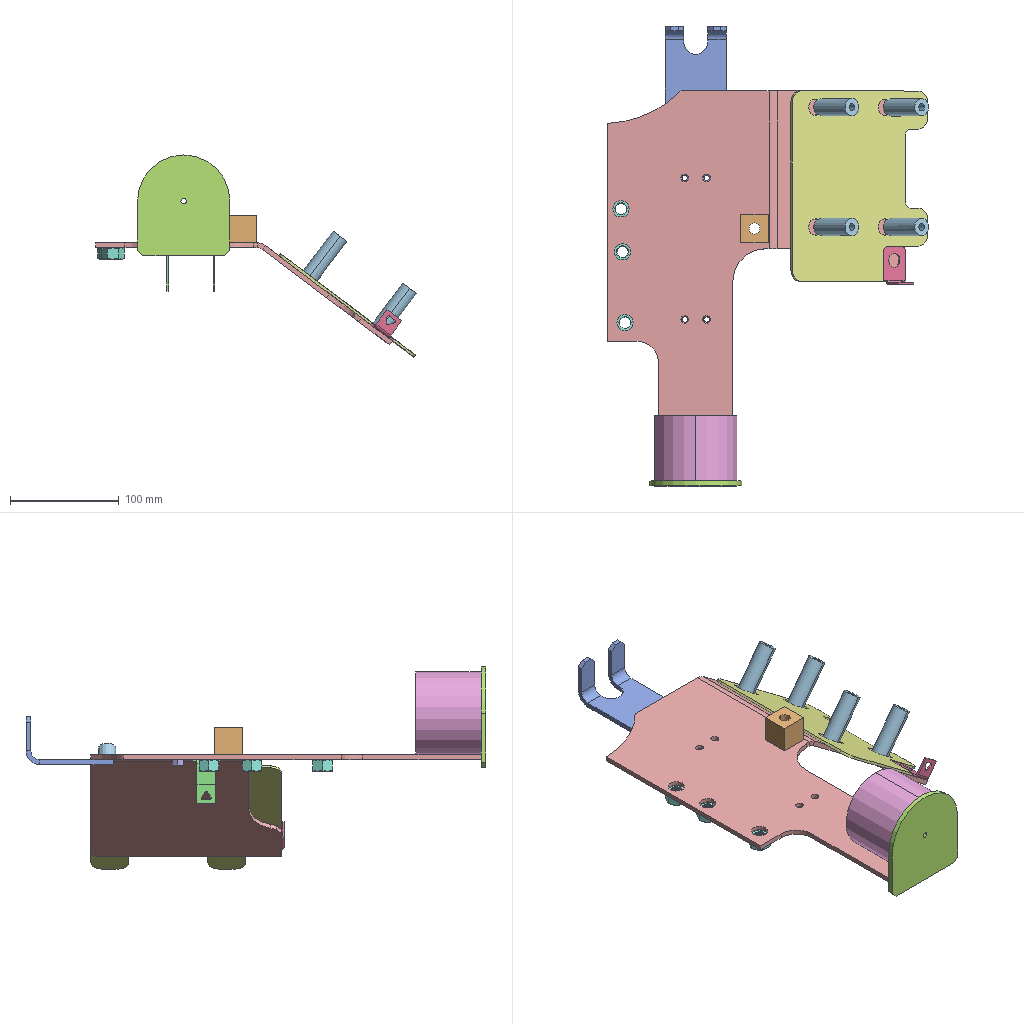Assembly | SolidWorks | 11 different items | 19 placed | box 295 x 422 x 186 mm
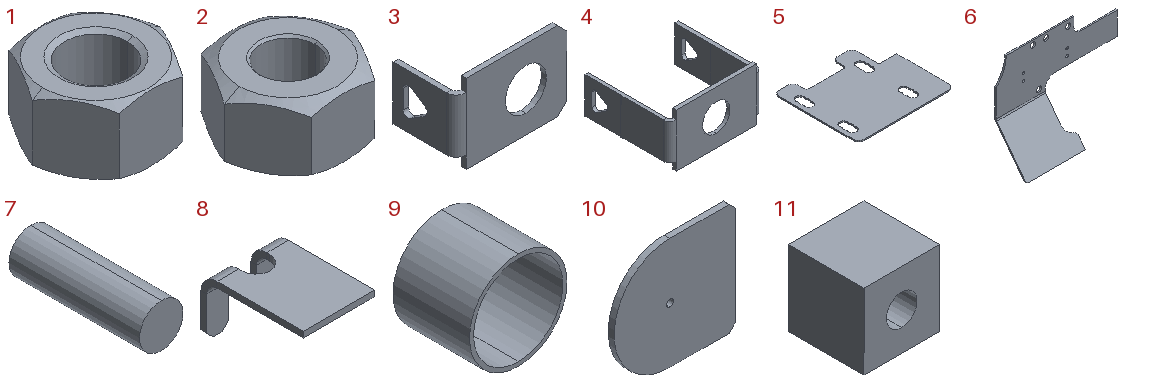Parts list (item | quantity | size | volume | features):
1 | x3 | 27.713 x 24 x 14.8 mm | 5071 mm3 | features RevCut 2, Chamfer 1, Extrusion 1, LPattern 1
2 | x4 | 11.547 x 10 x 5.7 mm | 373.519 mm3 | features RevCut 4, Chamfer 2, Boss 1, Extrusion 1, LPattern 1
3 | x1 | 35 x 20 x 25 mm | 1534 mm3 | features ICE 2, Chamfer 1, FlatPattern 1, SMBaseFlange 1, SheetMetal 1
4 | x1 | 44 x 40 x 25 mm | 3354 mm3 | features ICE 6, FlatPattern 1, MirrorPattern 1, SMBaseFlange 1, SheetMetal 1
5 | x1 | 175 x 155 x 2.3 mm | 50413 mm3 | features FlatPattern 1, SMBaseFlange 1, SheetMetal 1
6 | x1 | 358.5 x 93.6 x 272.5 mm | 277136 mm3 | features ICE 2, Chamfer 1, FlatPattern 1, SMBaseFlange 1, SheetMetal 1
7 | x4 | 16 x 48 x 16 mm | 8682 mm3 | features Extrusion 1, HoleWzd 1
8 | x1 | 56 x 80 x 44 mm | 22975 mm3 | features Chamfer 1, FlatPattern 1, ICE 1, SMBaseFlange 1, SheetMetal 1
9 | x1 | 76.3 x 60 x 76.3 mm | 44093 mm3 | features Extrusion 1
10 | x1 | 92.5 x 4.5 x 85 mm | 31692 mm3 | features FlatPattern 1, SMBaseFlange 1, SheetMetal 1
11 | x1 | 25 x 25 x 25 mm | 13582 mm3 | features Extrusion 1, HoleWzd 1
Mates (type | each side: item.copy, entity, surface, feature):
Coincident | 6.1 face plane Base-Flange1 | 8.1 face plane Base-Flange1
DistanceDim | 8.1 face plane Base-Flange1 | 6.1 face plane Base-Flange1 | 2 times
Coincident | 6.1 face plane Base-Flange1 | 10.1 face plane Base-Flange1
DistanceDim | 10.1 face cylinder Base-Flange1 | 6.1 face plane Base-Flange1
DistanceDim | 6.1 face plane Cut-Extrude1 | 10.1 face plane Base-Flange1
Concentric | 10.1 face cylinder Base-Flange1 | 9.1 face cylinder Boss-Extrude1
Parallel | 9.1 plane | assembly plane
Coincident | 10.1 face plane Base-Flange1 | 9.1 face plane Boss-Extrude1
Concentric | 6.1 face cylinder Cut-Extrude1 | 1.1 face cone EndChamfer
Coincident | 6.1 face plane Base-Flange1 | 1.1 face plane BaseNut
Concentric | 6.1 face cylinder Cut-Extrude1 | 1.2 face cone EndChamfer
Coincident | 6.1 face plane Base-Flange1 | 1.2 face plane BaseNut
Concentric | 6.1 face cylinder Cut-Extrude1 | 1.3 face cone EndChamfer
Coincident | 6.1 face plane Base-Flange1 | 1.3 face plane BaseNut
Concentric | 6.1 face cylinder Cut-Extrude1 | 11.1 face cylinder M12 Tapped Hole1
Coincident | 6.1 face plane Base-Flange1 | 11.1 face plane Boss-Extrude1
Parallel | 6.1 face plane Base-Flange1 | 11.1 face plane Boss-Extrude1
Parallel | 6.1 face plane Cut-Extrude1 | 1.1 face plane BaseNut
Parallel | 6.1 face plane Cut-Extrude1 | 1.2 face plane BaseNut
Parallel | 6.1 face plane Cut-Extrude1 | 1.3 face plane BaseNut
Concentric | 6.1 face cylinder Cut-Extrude1 | 2.1 face cone EndChamfer1
Coincident | 6.1 face plane Base-Flange1 | 2.1 face plane BaseNut
Concentric | 6.1 face cylinder Cut-Extrude1 | 2.2 face cone EndChamfer1
Coincident | 6.1 face plane Base-Flange1 | 2.2 face plane BaseNut
Parallel | 6.1 face plane Cut-Extrude1 | 2.2 face plane BaseNut
Parallel | 6.1 face plane Cut-Extrude1 | 2.1 face plane BaseNut
Coincident | 6.1 face plane Base-Flange1 | 4.1 face plane Base-Flange1
DistanceDim | 4.1 face plane Base-Flange1 | 6.1 face plane Base-Flange1 | 2 times
Coincident | 6.1 face plane Base-Flange1 | 3.1 face plane Base-Flange1 | 2 times
DistanceDim | 3.1 face plane Base-Flange1 | 6.1 face plane Base-Flange1
Coincident | 6.1 face plane Base-Flange1 | 7.1 face plane Boss-Extrude1
DistanceDim | 7.1 face cylinder Boss-Extrude1 | 6.1 face plane Base-Flange1
DistanceDim | 6.1 face plane Base-Flange1 | 7.1 face cylinder Boss-Extrude1
Parallel | 6.1 face plane Base-Flange1 | 7.1 plane
Concentric | 7.1 face cylinder Boss-Extrude1 | 5.1 face cylinder Base-Flange1
Concentric | 7.2 face cylinder Boss-Extrude1 | 5.1 face cylinder Base-Flange1
Coincident | 6.1 face plane Base-Flange1 | 5.1 face plane Base-Flange1